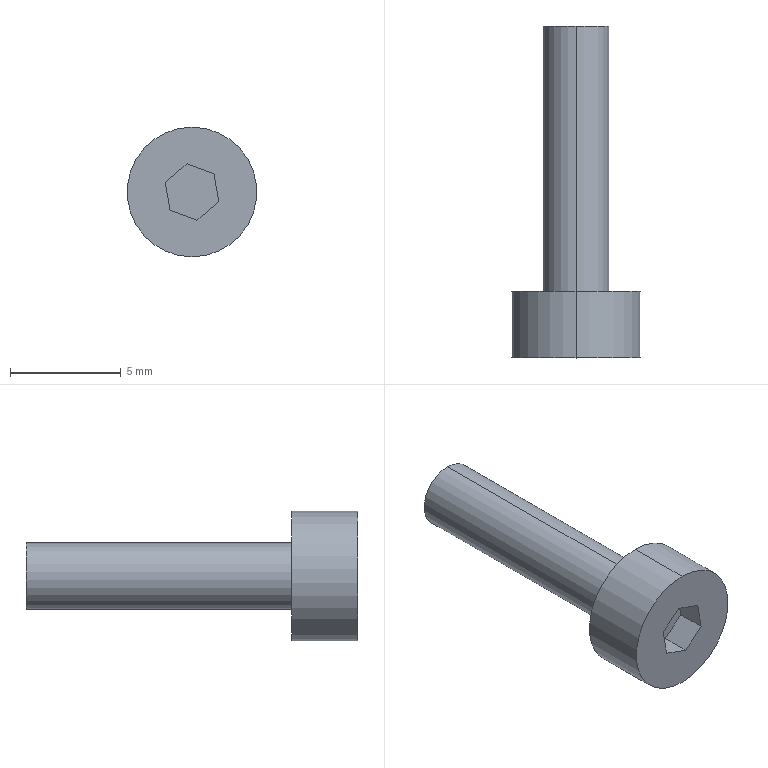Part | SolidWorks | features ICE 2, Extrusion 1 | 1 solid | 14 faces | box 5.86 x 15 x 5.86 mm | volume 160.113 mm3 | plane 10 | cylinder 4 | commonest cylinder face diameters 3 x2 5.86 x2
STEP:
#1=CARTESIAN_POINT('',(0.,15.,1.5));
#2=VERTEX_POINT('',#1);
#3=CARTESIAN_POINT('',(0.,15.,-1.5));
#4=VERTEX_POINT('',#3);
#5=CARTESIAN_POINT('',(0.,15.,0.));
#6=DIRECTION('',(0.,1.,0.));
#7=DIRECTION('',(0.,0.,1.));
#8=AXIS2_PLACEMENT_3D('',#5,#6,#7);
#9=CIRCLE('',#8,1.5);
#10=EDGE_CURVE('',#2,#4,#9,.T.);
#11=ORIENTED_EDGE('',*,*,#10,.F.);
#12=CARTESIAN_POINT('',(0.,3.,1.5));
#13=VERTEX_POINT('',#12);
#14=CARTESIAN_POINT('',(0.,15.,1.5));
#15=DIRECTION('',(0.,-1.,0.));
#16=VECTOR('',#15,1000.);
#17=LINE('',#14,#16);
#18=EDGE_CURVE('',#2,#13,#17,.T.);
#19=ORIENTED_EDGE('',*,*,#18,.T.);
#20=CARTESIAN_POINT('',(0.,3.,-1.5));
#21=VERTEX_POINT('',#20);
#22=CARTESIAN_POINT('',(0.,3.,0.));
#23=DIRECTION('',(0.,1.,0.));
#24=DIRECTION('',(0.,0.,1.));
#25=AXIS2_PLACEMENT_3D('',#22,#23,#24);
#26=CIRCLE('',#25,1.5);
#27=EDGE_CURVE('',#13,#21,#26,.T.);
#28=ORIENTED_EDGE('',*,*,#27,.T.);
#29=CARTESIAN_POINT('',(0.,15.,-1.5));
#30=DIRECTION('',(0.,-1.,0.));
#31=VECTOR('',#30,1000.);
#32=LINE('',#29,#31);
#33=EDGE_CURVE('',#4,#21,#32,.T.);
#34=ORIENTED_EDGE('',*,*,#33,.F.);
#35=EDGE_LOOP('',(#11,#19,#28,#34));
#36=FACE_OUTER_BOUND('',#35,.T.);
#37=CARTESIAN_POINT('',(0.,15.,0.));
#38=DIRECTION('',(0.,-1.,0.));
#39=DIRECTION('',(0.,0.,-1.));
#40=AXIS2_PLACEMENT_3D('',#37,#38,#39);
#41=CYLINDRICAL_SURFACE('',#40,1.5);
#42=ADVANCED_FACE('',(#36),#41,.T.);
#43=CARTESIAN_POINT('',(0.,3.,2.93));
#44=VERTEX_POINT('',#43);
#45=CARTESIAN_POINT('',(0.,3.,-2.93));
#46=VERTEX_POINT('',#45);
#47=CARTESIAN_POINT('',(0.,3.,0.));
#48=DIRECTION('',(0.,1.,0.));
#49=DIRECTION('',(0.,0.,1.));
#50=AXIS2_PLACEMENT_3D('',#47,#48,#49);
#51=CIRCLE('',#50,2.93);
#52=EDGE_CURVE('',#44,#46,#51,.T.);
#53=ORIENTED_EDGE('',*,*,#52,.F.);
#54=CARTESIAN_POINT('',(0.,0.,2.93));
#55=VERTEX_POINT('',#54);
#56=CARTESIAN_POINT('',(0.,3.,2.93));
#57=DIRECTION('',(0.,-1.,0.));
#58=VECTOR('',#57,1000.);
#59=LINE('',#56,#58);
#60=EDGE_CURVE('',#44,#55,#59,.T.);
#61=ORIENTED_EDGE('',*,*,#60,.T.);
#62=CARTESIAN_POINT('',(0.,0.,-2.93));
#63=VERTEX_POINT('',#62);
#64=CARTESIAN_POINT('',(0.,0.,0.));
#65=DIRECTION('',(0.,1.,0.));
#66=DIRECTION('',(0.,0.,1.));
#67=AXIS2_PLACEMENT_3D('',#64,#65,#66);
#68=CIRCLE('',#67,2.93);
#69=EDGE_CURVE('',#55,#63,#68,.T.);
#70=ORIENTED_EDGE('',*,*,#69,.T.);
#71=CARTESIAN_POINT('',(0.,3.,-2.93));
#72=DIRECTION('',(0.,-1.,0.));
#73=VECTOR('',#72,1000.);
#74=LINE('',#71,#73);
#75=EDGE_CURVE('',#46,#63,#74,.T.);
#76=ORIENTED_EDGE('',*,*,#75,.F.);
#77=EDGE_LOOP('',(#53,#61,#70,#76));
#78=FACE_OUTER_BOUND('',#77,.T.);
#79=CARTESIAN_POINT('',(0.,3.,0.));
#80=DIRECTION('',(0.,-1.,0.));
#81=DIRECTION('',(0.,0.,-1.));
#82=AXIS2_PLACEMENT_3D('',#79,#80,#81);
#83=CYLINDRICAL_SURFACE('',#82,2.93);
#84=ADVANCED_FACE('',(#78),#83,.T.);
#85=ORIENTED_EDGE('',*,*,#60,.F.);
#86=CARTESIAN_POINT('',(0.,3.,0.));
#87=DIRECTION('',(0.,1.,0.));
#88=DIRECTION('',(0.,0.,1.));
#89=AXIS2_PLACEMENT_3D('',#86,#87,#88);
#90=CIRCLE('',#89,2.93);
#91=EDGE_CURVE('',#46,#44,#90,.T.);
#92=ORIENTED_EDGE('',*,*,#91,.F.);
#93=ORIENTED_EDGE('',*,*,#75,.T.);
#94=CARTESIAN_POINT('',(0.,0.,0.));
#95=DIRECTION('',(0.,1.,0.));
#96=DIRECTION('',(0.,0.,1.));
#97=AXIS2_PLACEMENT_3D('',#94,#95,#96);
#98=CIRCLE('',#97,2.93);
#99=EDGE_CURVE('',#63,#55,#98,.T.);
#100=ORIENTED_EDGE('',*,*,#99,.T.);
#101=EDGE_LOOP('',(#85,#92,#93,#100));
#102=FACE_OUTER_BOUND('',#101,.T.);
#103=CARTESIAN_POINT('',(0.,3.,0.));
#104=DIRECTION('',(0.,-1.,0.));
#105=DIRECTION('',(0.,0.,-1.));
#106=AXIS2_PLACEMENT_3D('',#103,#104,#105);
#107=CYLINDRICAL_SURFACE('',#106,2.93);
#108=ADVANCED_FACE('',(#102),#107,.T.);
#109=CARTESIAN_POINT('',(0.,3.,0.));
#110=DIRECTION('',(0.,1.,0.));
#111=DIRECTION('',(0.,0.,1.));
#112=AXIS2_PLACEMENT_3D('',#109,#110,#111);
#113=CIRCLE('',#112,1.5);
#114=EDGE_CURVE('',#21,#13,#113,.T.);
#115=ORIENTED_EDGE('',*,*,#114,.F.);
#116=ORIENTED_EDGE('',*,*,#27,.F.);
#117=EDGE_LOOP('',(#115,#116));
#118=FACE_BOUND('',#117,.T.);
#119=ORIENTED_EDGE('',*,*,#91,.T.);
#120=ORIENTED_EDGE('',*,*,#52,.T.);
#121=EDGE_LOOP('',(#119,#120));
#122=FACE_OUTER_BOUND('',#121,.T.);
#123=CARTESIAN_POINT('',(0.,3.,0.));
#124=DIRECTION('',(0.,1.,0.));
#125=DIRECTION('',(0.,0.,1.));
#126=AXIS2_PLACEMENT_3D('',#123,#124,#125);
#127=PLANE('',#126);
#128=ADVANCED_FACE('',(#118,#122),#127,.T.);
#129=CARTESIAN_POINT('',(0.9898,0.,0.8273));
#130=VERTEX_POINT('',#129);
#131=CARTESIAN_POINT('',(-0.2216,0.,1.271));
#132=VERTEX_POINT('',#131);
#133=CARTESIAN_POINT('',(0.9898,0.,0.8273));
#134=DIRECTION('',(-0.939,0.,0.3438));
#135=VECTOR('',#134,1000.);
#136=LINE('',#133,#135);
#137=EDGE_CURVE('',#130,#132,#136,.T.);
#138=ORIENTED_EDGE('',*,*,#137,.F.);
#139=CARTESIAN_POINT('',(1.211,0.,-0.4435));
#140=VERTEX_POINT('',#139);
#141=CARTESIAN_POINT('',(1.211,0.,-0.4435));
#142=DIRECTION('',(-0.1718,0.,0.9851));
#143=VECTOR('',#142,1000.);
#144=LINE('',#141,#143);
#145=EDGE_CURVE('',#140,#130,#144,.T.);
#146=ORIENTED_EDGE('',*,*,#145,.F.);
#147=CARTESIAN_POINT('',(0.2216,0.,-1.271));
#148=VERTEX_POINT('',#147);
#149=CARTESIAN_POINT('',(0.2216,0.,-1.271));
#150=DIRECTION('',(0.7673,0.,0.6413));
#151=VECTOR('',#150,1000.);
#152=LINE('',#149,#151);
#153=EDGE_CURVE('',#148,#140,#152,.T.);
#154=ORIENTED_EDGE('',*,*,#153,.F.);
#155=CARTESIAN_POINT('',(-0.9898,0.,-0.8273));
#156=VERTEX_POINT('',#155);
#157=CARTESIAN_POINT('',(-0.9898,0.,-0.8273));
#158=DIRECTION('',(0.939,0.,-0.3438));
#159=VECTOR('',#158,1000.);
#160=LINE('',#157,#159);
#161=EDGE_CURVE('',#156,#148,#160,.T.);
#162=ORIENTED_EDGE('',*,*,#161,.F.);
#163=CARTESIAN_POINT('',(-1.211,0.,0.4435));
#164=VERTEX_POINT('',#163);
#165=CARTESIAN_POINT('',(-1.211,0.,0.4435));
#166=DIRECTION('',(0.1718,0.,-0.9851));
#167=VECTOR('',#166,1000.);
#168=LINE('',#165,#167);
#169=EDGE_CURVE('',#164,#156,#168,.T.);
#170=ORIENTED_EDGE('',*,*,#169,.F.);
#171=CARTESIAN_POINT('',(-0.2216,0.,1.271));
#172=DIRECTION('',(-0.7673,0.,-0.6413));
#173=VECTOR('',#172,1000.);
#174=LINE('',#171,#173);
#175=EDGE_CURVE('',#132,#164,#174,.T.);
#176=ORIENTED_EDGE('',*,*,#175,.F.);
#177=EDGE_LOOP('',(#138,#146,#154,#162,#170,#176));
#178=FACE_BOUND('',#177,.T.);
#179=ORIENTED_EDGE('',*,*,#99,.F.);
#180=ORIENTED_EDGE('',*,*,#69,.F.);
#181=EDGE_LOOP('',(#179,#180));
#182=FACE_OUTER_BOUND('',#181,.T.);
#183=CARTESIAN_POINT('',(0.,0.,0.));
#184=DIRECTION('',(0.,1.,0.));
#185=DIRECTION('',(0.,0.,1.));
#186=AXIS2_PLACEMENT_3D('',#183,#184,#185);
#187=PLANE('',#186);
#188=ADVANCED_FACE('',(#178,#182),#187,.F.);
#189=ORIENTED_EDGE('',*,*,#18,.F.);
#190=CARTESIAN_POINT('',(0.,15.,0.));
#191=DIRECTION('',(0.,1.,0.));
#192=DIRECTION('',(0.,0.,1.));
#193=AXIS2_PLACEMENT_3D('',#190,#191,#192);
#194=CIRCLE('',#193,1.5);
#195=EDGE_CURVE('',#4,#2,#194,.T.);
#196=ORIENTED_EDGE('',*,*,#195,.F.);
#197=ORIENTED_EDGE('',*,*,#33,.T.);
#198=ORIENTED_EDGE('',*,*,#114,.T.);
#199=EDGE_LOOP('',(#189,#196,#197,#198));
#200=FACE_OUTER_BOUND('',#199,.T.);
#201=CARTESIAN_POINT('',(0.,15.,0.));
#202=DIRECTION('',(0.,-1.,0.));
#203=DIRECTION('',(0.,0.,-1.));
#204=AXIS2_PLACEMENT_3D('',#201,#202,#203);
#205=CYLINDRICAL_SURFACE('',#204,1.5);
#206=ADVANCED_FACE('',(#200),#205,.T.);
#207=ORIENTED_EDGE('',*,*,#195,.T.);
#208=ORIENTED_EDGE('',*,*,#10,.T.);
#209=EDGE_LOOP('',(#207,#208));
#210=FACE_OUTER_BOUND('',#209,.T.);
#211=CARTESIAN_POINT('',(0.,15.,0.));
#212=DIRECTION('',(0.,1.,0.));
#213=DIRECTION('',(0.,0.,1.));
#214=AXIS2_PLACEMENT_3D('',#211,#212,#213);
#215=PLANE('',#214);
#216=ADVANCED_FACE('',(#210),#215,.T.);
#217=ORIENTED_EDGE('',*,*,#145,.T.);
#218=CARTESIAN_POINT('',(0.9898,1.3,0.8273));
#219=VERTEX_POINT('',#218);
#220=CARTESIAN_POINT('',(0.9898,1.3,0.8273));
#221=DIRECTION('',(0.,-1.,0.));
#222=VECTOR('',#221,1000.);
#223=LINE('',#220,#222);
#224=EDGE_CURVE('',#219,#130,#223,.T.);
#225=ORIENTED_EDGE('',*,*,#224,.F.);
#226=CARTESIAN_POINT('',(1.211,1.3,-0.4435));
#227=VERTEX_POINT('',#226);
#228=CARTESIAN_POINT('',(1.211,1.3,-0.4435));
#229=DIRECTION('',(-0.1718,0.,0.9851));
#230=VECTOR('',#229,1000.);
#231=LINE('',#228,#230);
#232=EDGE_CURVE('',#227,#219,#231,.T.);
#233=ORIENTED_EDGE('',*,*,#232,.F.);
#234=CARTESIAN_POINT('',(1.211,1.3,-0.4435));
#235=DIRECTION('',(0.,-1.,0.));
#236=VECTOR('',#235,1000.);
#237=LINE('',#234,#236);
#238=EDGE_CURVE('',#227,#140,#237,.T.);
#239=ORIENTED_EDGE('',*,*,#238,.T.);
#240=EDGE_LOOP('',(#217,#225,#233,#239));
#241=FACE_OUTER_BOUND('',#240,.T.);
#242=CARTESIAN_POINT('',(1.211,1.3,-0.4435));
#243=DIRECTION('',(0.9851,0.,0.1718));
#244=DIRECTION('',(0.1718,0.,-0.9851));
#245=AXIS2_PLACEMENT_3D('',#242,#243,#244);
#246=PLANE('',#245);
#247=ADVANCED_FACE('',(#241),#246,.F.);
#248=ORIENTED_EDGE('',*,*,#153,.T.);
#249=ORIENTED_EDGE('',*,*,#238,.F.);
#250=CARTESIAN_POINT('',(0.2216,1.3,-1.271));
#251=VERTEX_POINT('',#250);
#252=CARTESIAN_POINT('',(0.2216,1.3,-1.271));
#253=DIRECTION('',(0.7673,0.,0.6413));
#254=VECTOR('',#253,1000.);
#255=LINE('',#252,#254);
#256=EDGE_CURVE('',#251,#227,#255,.T.);
#257=ORIENTED_EDGE('',*,*,#256,.F.);
#258=CARTESIAN_POINT('',(0.2216,1.3,-1.271));
#259=DIRECTION('',(0.,-1.,0.));
#260=VECTOR('',#259,1000.);
#261=LINE('',#258,#260);
#262=EDGE_CURVE('',#251,#148,#261,.T.);
#263=ORIENTED_EDGE('',*,*,#262,.T.);
#264=EDGE_LOOP('',(#248,#249,#257,#263));
#265=FACE_OUTER_BOUND('',#264,.T.);
#266=CARTESIAN_POINT('',(0.2216,1.3,-1.271));
#267=DIRECTION('',(0.6413,0.,-0.7673));
#268=DIRECTION('',(-0.7673,0.,-0.6413));
#269=AXIS2_PLACEMENT_3D('',#266,#267,#268);
#270=PLANE('',#269);
#271=ADVANCED_FACE('',(#265),#270,.F.);
#272=ORIENTED_EDGE('',*,*,#161,.T.);
#273=ORIENTED_EDGE('',*,*,#262,.F.);
#274=CARTESIAN_POINT('',(-0.9898,1.3,-0.8273));
#275=VERTEX_POINT('',#274);
#276=CARTESIAN_POINT('',(-0.9898,1.3,-0.8273));
#277=DIRECTION('',(0.939,0.,-0.3438));
#278=VECTOR('',#277,1000.);
#279=LINE('',#276,#278);
#280=EDGE_CURVE('',#275,#251,#279,.T.);
#281=ORIENTED_EDGE('',*,*,#280,.F.);
#282=CARTESIAN_POINT('',(-0.9898,1.3,-0.8273));
#283=DIRECTION('',(0.,-1.,0.));
#284=VECTOR('',#283,1000.);
#285=LINE('',#282,#284);
#286=EDGE_CURVE('',#275,#156,#285,.T.);
#287=ORIENTED_EDGE('',*,*,#286,.T.);
#288=EDGE_LOOP('',(#272,#273,#281,#287));
#289=FACE_OUTER_BOUND('',#288,.T.);
#290=CARTESIAN_POINT('',(-0.9898,1.3,-0.8273));
#291=DIRECTION('',(-0.3438,0.,-0.939));
#292=DIRECTION('',(-0.939,0.,0.3438));
#293=AXIS2_PLACEMENT_3D('',#290,#291,#292);
#294=PLANE('',#293);
#295=ADVANCED_FACE('',(#289),#294,.F.);
#296=ORIENTED_EDGE('',*,*,#169,.T.);
#297=ORIENTED_EDGE('',*,*,#286,.F.);
#298=CARTESIAN_POINT('',(-1.211,1.3,0.4435));
#299=VERTEX_POINT('',#298);
#300=CARTESIAN_POINT('',(-1.211,1.3,0.4435));
#301=DIRECTION('',(0.1718,0.,-0.9851));
#302=VECTOR('',#301,1000.);
#303=LINE('',#300,#302);
#304=EDGE_CURVE('',#299,#275,#303,.T.);
#305=ORIENTED_EDGE('',*,*,#304,.F.);
#306=CARTESIAN_POINT('',(-1.211,1.3,0.4435));
#307=DIRECTION('',(0.,-1.,0.));
#308=VECTOR('',#307,1000.);
#309=LINE('',#306,#308);
#310=EDGE_CURVE('',#299,#164,#309,.T.);
#311=ORIENTED_EDGE('',*,*,#310,.T.);
#312=EDGE_LOOP('',(#296,#297,#305,#311));
#313=FACE_OUTER_BOUND('',#312,.T.);
#314=CARTESIAN_POINT('',(-1.211,1.3,0.4435));
#315=DIRECTION('',(-0.9851,0.,-0.1718));
#316=DIRECTION('',(-0.1718,0.,0.9851));
#317=AXIS2_PLACEMENT_3D('',#314,#315,#316);
#318=PLANE('',#317);
#319=ADVANCED_FACE('',(#313),#318,.F.);
#320=ORIENTED_EDGE('',*,*,#175,.T.);
#321=ORIENTED_EDGE('',*,*,#310,.F.);
#322=CARTESIAN_POINT('',(-0.2216,1.3,1.271));
#323=VERTEX_POINT('',#322);
#324=CARTESIAN_POINT('',(-0.2216,1.3,1.271));
#325=DIRECTION('',(-0.7673,0.,-0.6413));
#326=VECTOR('',#325,1000.);
#327=LINE('',#324,#326);
#328=EDGE_CURVE('',#323,#299,#327,.T.);
#329=ORIENTED_EDGE('',*,*,#328,.F.);
#330=CARTESIAN_POINT('',(-0.2216,1.3,1.271));
#331=DIRECTION('',(0.,-1.,0.));
#332=VECTOR('',#331,1000.);
#333=LINE('',#330,#332);
#334=EDGE_CURVE('',#323,#132,#333,.T.);
#335=ORIENTED_EDGE('',*,*,#334,.T.);
#336=EDGE_LOOP('',(#320,#321,#329,#335));
#337=FACE_OUTER_BOUND('',#336,.T.);
#338=CARTESIAN_POINT('',(-0.2216,1.3,1.271));
#339=DIRECTION('',(-0.6413,0.,0.7673));
#340=DIRECTION('',(0.7673,0.,0.6413));
#341=AXIS2_PLACEMENT_3D('',#338,#339,#340);
#342=PLANE('',#341);
#343=ADVANCED_FACE('',(#337),#342,.F.);
#344=ORIENTED_EDGE('',*,*,#137,.T.);
#345=ORIENTED_EDGE('',*,*,#334,.F.);
#346=CARTESIAN_POINT('',(0.9898,1.3,0.8273));
#347=DIRECTION('',(-0.939,0.,0.3438));
#348=VECTOR('',#347,1000.);
#349=LINE('',#346,#348);
#350=EDGE_CURVE('',#219,#323,#349,.T.);
#351=ORIENTED_EDGE('',*,*,#350,.F.);
#352=ORIENTED_EDGE('',*,*,#224,.T.);
#353=EDGE_LOOP('',(#344,#345,#351,#352));
#354=FACE_OUTER_BOUND('',#353,.T.);
#355=CARTESIAN_POINT('',(0.9898,1.3,0.8273));
#356=DIRECTION('',(0.3438,0.,0.939));
#357=DIRECTION('',(0.939,0.,-0.3438));
#358=AXIS2_PLACEMENT_3D('',#355,#356,#357);
#359=PLANE('',#358);
#360=ADVANCED_FACE('',(#354),#359,.F.);
#361=ORIENTED_EDGE('',*,*,#232,.T.);
#362=ORIENTED_EDGE('',*,*,#350,.T.);
#363=ORIENTED_EDGE('',*,*,#328,.T.);
#364=ORIENTED_EDGE('',*,*,#304,.T.);
#365=ORIENTED_EDGE('',*,*,#280,.T.);
#366=ORIENTED_EDGE('',*,*,#256,.T.);
#367=EDGE_LOOP('',(#361,#362,#363,#364,#365,#366));
#368=FACE_OUTER_BOUND('',#367,.T.);
#369=CARTESIAN_POINT('',(0.,1.3,0.));
#370=DIRECTION('',(0.,-1.,0.));
#371=DIRECTION('',(0.,0.,-1.));
#372=AXIS2_PLACEMENT_3D('',#369,#370,#371);
#373=PLANE('',#372);
#374=ADVANCED_FACE('',(#368),#373,.T.);
#375=CLOSED_SHELL('',(#42,#84,#108,#128,#188,#206,#216,#247,#271,#295,#319,#343,#360,#374));
#376=MANIFOLD_SOLID_BREP('',#375);
#377=CARTESIAN_POINT('',(0.,0.,0.));
#378=DIRECTION('',(0.,0.,1.));
#379=DIRECTION('',(1.,0.,0.));
#380=AXIS2_PLACEMENT_3D('',#377,#378,#379);
#381=(LENGTH_UNIT()NAMED_UNIT(*)SI_UNIT(.MILLI.,.METRE.));
#382=UNCERTAINTY_MEASURE_WITH_UNIT(LENGTH_MEASURE(0.00001),#381,'','');
#383=(NAMED_UNIT(*)PLANE_ANGLE_UNIT()SI_UNIT($,.RADIAN.));
#384=(NAMED_UNIT(*)SI_UNIT($,.STERADIAN.)SOLID_ANGLE_UNIT());
#385=(GEOMETRIC_REPRESENTATION_CONTEXT(3)GLOBAL_UNCERTAINTY_ASSIGNED_CONTEXT((#382))GLOBAL_UNIT_ASSIGNED_CONTEXT((#381,#383,#384))REPRESENTATION_CONTEXT('',''));
#386=ADVANCED_BREP_SHAPE_REPRESENTATION('',(#376,#380),#385);